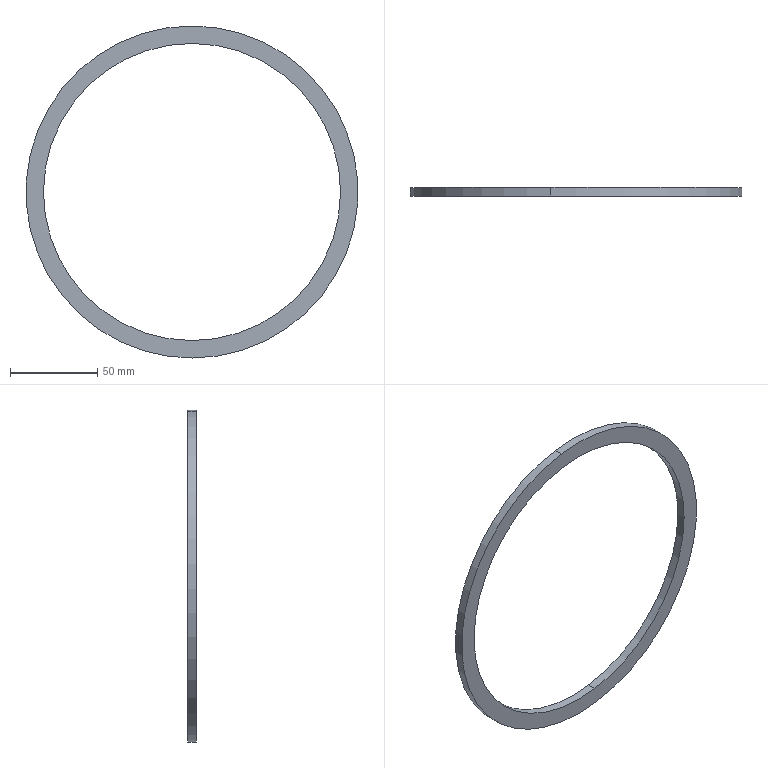Part | STEP file | 2026.6.15-Main Assembly图.sldasm-Part-10 | 1 solid | 6 faces | box 190 x 5 x 190 mm | volume 28274 mm3 | cylinder 4 | plane 2 | commonest cylinder face diameters 170 x2 190 x2
STEP:
#1=CARTESIAN_POINT('',(-741.485,695.541,3110.617));
#2=VERTEX_POINT('',#1);
#3=CARTESIAN_POINT('',(-767.19,695.541,3278.663));
#4=VERTEX_POINT('',#3);
#5=CARTESIAN_POINT('',(-754.337,695.541,3194.64));
#6=DIRECTION('',(0.,1.,0.));
#7=DIRECTION('',(-0.1512,0.,0.9885));
#8=AXIS2_PLACEMENT_3D('',#5,#6,#7);
#9=CIRCLE('',#8,85.);
#10=EDGE_CURVE('',#2,#4,#9,.T.);
#11=ORIENTED_EDGE('',*,*,#10,.T.);
#12=CARTESIAN_POINT('',(-767.19,690.541,3278.663));
#13=VERTEX_POINT('',#12);
#14=CARTESIAN_POINT('',(-767.19,695.541,3278.663));
#15=DIRECTION('',(0.,1.,0.));
#16=VECTOR('',#15,1000.);
#17=LINE('',#14,#16);
#18=EDGE_CURVE('',#13,#4,#17,.T.);
#19=ORIENTED_EDGE('',*,*,#18,.F.);
#20=CARTESIAN_POINT('',(-741.485,690.541,3110.617));
#21=VERTEX_POINT('',#20);
#22=CARTESIAN_POINT('',(-754.337,690.541,3194.64));
#23=DIRECTION('',(0.,1.,0.));
#24=DIRECTION('',(-0.1512,0.,0.9885));
#25=AXIS2_PLACEMENT_3D('',#22,#23,#24);
#26=CIRCLE('',#25,85.);
#27=EDGE_CURVE('',#21,#13,#26,.T.);
#28=ORIENTED_EDGE('',*,*,#27,.F.);
#29=CARTESIAN_POINT('',(-741.485,695.541,3110.617));
#30=DIRECTION('',(0.,1.,0.));
#31=VECTOR('',#30,1000.);
#32=LINE('',#29,#31);
#33=EDGE_CURVE('',#21,#2,#32,.T.);
#34=ORIENTED_EDGE('',*,*,#33,.T.);
#35=EDGE_LOOP('',(#11,#19,#28,#34));
#36=FACE_OUTER_BOUND('',#35,.T.);
#37=CARTESIAN_POINT('',(-754.337,695.541,3194.64));
#38=DIRECTION('',(0.,-1.,0.));
#39=DIRECTION('',(-0.1512,0.,0.9885));
#40=AXIS2_PLACEMENT_3D('',#37,#38,#39);
#41=CYLINDRICAL_SURFACE('',#40,85.);
#42=ADVANCED_FACE('',(#36),#41,.F.);
#43=CARTESIAN_POINT('',(-768.702,695.541,3288.548));
#44=VERTEX_POINT('',#43);
#45=CARTESIAN_POINT('',(-739.973,695.541,3100.732));
#46=VERTEX_POINT('',#45);
#47=CARTESIAN_POINT('',(-754.337,695.541,3194.64));
#48=DIRECTION('',(0.,1.,0.));
#49=DIRECTION('',(-0.1512,0.,0.9885));
#50=AXIS2_PLACEMENT_3D('',#47,#48,#49);
#51=CIRCLE('',#50,95.);
#52=EDGE_CURVE('',#44,#46,#51,.T.);
#53=ORIENTED_EDGE('',*,*,#52,.F.);
#54=CARTESIAN_POINT('',(-768.702,690.541,3288.548));
#55=VERTEX_POINT('',#54);
#56=CARTESIAN_POINT('',(-768.702,695.541,3288.548));
#57=DIRECTION('',(0.,1.,0.));
#58=VECTOR('',#57,1000.);
#59=LINE('',#56,#58);
#60=EDGE_CURVE('',#55,#44,#59,.T.);
#61=ORIENTED_EDGE('',*,*,#60,.F.);
#62=CARTESIAN_POINT('',(-739.973,690.541,3100.732));
#63=VERTEX_POINT('',#62);
#64=CARTESIAN_POINT('',(-754.337,690.541,3194.64));
#65=DIRECTION('',(0.,1.,0.));
#66=DIRECTION('',(-0.1512,0.,0.9885));
#67=AXIS2_PLACEMENT_3D('',#64,#65,#66);
#68=CIRCLE('',#67,95.);
#69=EDGE_CURVE('',#55,#63,#68,.T.);
#70=ORIENTED_EDGE('',*,*,#69,.T.);
#71=CARTESIAN_POINT('',(-739.973,695.541,3100.732));
#72=DIRECTION('',(0.,1.,0.));
#73=VECTOR('',#72,1000.);
#74=LINE('',#71,#73);
#75=EDGE_CURVE('',#63,#46,#74,.T.);
#76=ORIENTED_EDGE('',*,*,#75,.T.);
#77=EDGE_LOOP('',(#53,#61,#70,#76));
#78=FACE_OUTER_BOUND('',#77,.T.);
#79=CARTESIAN_POINT('',(-754.337,695.541,3194.64));
#80=DIRECTION('',(0.,-1.,0.));
#81=DIRECTION('',(-0.1512,0.,0.9885));
#82=AXIS2_PLACEMENT_3D('',#79,#80,#81);
#83=CYLINDRICAL_SURFACE('',#82,95.);
#84=ADVANCED_FACE('',(#78),#83,.T.);
#85=CARTESIAN_POINT('',(-754.337,695.541,3194.64));
#86=DIRECTION('',(0.,1.,0.));
#87=DIRECTION('',(-0.1512,0.,0.9885));
#88=AXIS2_PLACEMENT_3D('',#85,#86,#87);
#89=CIRCLE('',#88,95.);
#90=EDGE_CURVE('',#46,#44,#89,.T.);
#91=ORIENTED_EDGE('',*,*,#90,.T.);
#92=ORIENTED_EDGE('',*,*,#52,.T.);
#93=EDGE_LOOP('',(#91,#92));
#94=FACE_OUTER_BOUND('',#93,.T.);
#95=ORIENTED_EDGE('',*,*,#10,.F.);
#96=CARTESIAN_POINT('',(-754.337,695.541,3194.64));
#97=DIRECTION('',(0.,1.,0.));
#98=DIRECTION('',(-0.1512,0.,0.9885));
#99=AXIS2_PLACEMENT_3D('',#96,#97,#98);
#100=CIRCLE('',#99,85.);
#101=EDGE_CURVE('',#4,#2,#100,.T.);
#102=ORIENTED_EDGE('',*,*,#101,.F.);
#103=EDGE_LOOP('',(#95,#102));
#104=FACE_BOUND('',#103,.T.);
#105=CARTESIAN_POINT('',(-754.337,695.541,3194.64));
#106=DIRECTION('',(0.,1.,0.));
#107=DIRECTION('',(0.1512,0.,-0.9885));
#108=AXIS2_PLACEMENT_3D('',#105,#106,#107);
#109=PLANE('',#108);
#110=ADVANCED_FACE('',(#94,#104),#109,.T.);
#111=CARTESIAN_POINT('',(-754.337,690.541,3194.64));
#112=DIRECTION('',(0.,1.,0.));
#113=DIRECTION('',(-0.1512,0.,0.9885));
#114=AXIS2_PLACEMENT_3D('',#111,#112,#113);
#115=CIRCLE('',#114,95.);
#116=EDGE_CURVE('',#63,#55,#115,.T.);
#117=ORIENTED_EDGE('',*,*,#116,.F.);
#118=ORIENTED_EDGE('',*,*,#69,.F.);
#119=EDGE_LOOP('',(#117,#118));
#120=FACE_OUTER_BOUND('',#119,.T.);
#121=ORIENTED_EDGE('',*,*,#27,.T.);
#122=CARTESIAN_POINT('',(-754.337,690.541,3194.64));
#123=DIRECTION('',(0.,1.,0.));
#124=DIRECTION('',(-0.1512,0.,0.9885));
#125=AXIS2_PLACEMENT_3D('',#122,#123,#124);
#126=CIRCLE('',#125,85.);
#127=EDGE_CURVE('',#13,#21,#126,.T.);
#128=ORIENTED_EDGE('',*,*,#127,.T.);
#129=EDGE_LOOP('',(#121,#128));
#130=FACE_BOUND('',#129,.T.);
#131=CARTESIAN_POINT('',(-754.337,690.541,3194.64));
#132=DIRECTION('',(0.,1.,0.));
#133=DIRECTION('',(0.1512,0.,-0.9885));
#134=AXIS2_PLACEMENT_3D('',#131,#132,#133);
#135=PLANE('',#134);
#136=ADVANCED_FACE('',(#120,#130),#135,.F.);
#137=ORIENTED_EDGE('',*,*,#60,.T.);
#138=ORIENTED_EDGE('',*,*,#90,.F.);
#139=ORIENTED_EDGE('',*,*,#75,.F.);
#140=ORIENTED_EDGE('',*,*,#116,.T.);
#141=EDGE_LOOP('',(#137,#138,#139,#140));
#142=FACE_OUTER_BOUND('',#141,.T.);
#143=CARTESIAN_POINT('',(-754.337,695.541,3194.64));
#144=DIRECTION('',(0.,-1.,0.));
#145=DIRECTION('',(-0.1512,0.,0.9885));
#146=AXIS2_PLACEMENT_3D('',#143,#144,#145);
#147=CYLINDRICAL_SURFACE('',#146,95.);
#148=ADVANCED_FACE('',(#142),#147,.T.);
#149=ORIENTED_EDGE('',*,*,#18,.T.);
#150=ORIENTED_EDGE('',*,*,#101,.T.);
#151=ORIENTED_EDGE('',*,*,#33,.F.);
#152=ORIENTED_EDGE('',*,*,#127,.F.);
#153=EDGE_LOOP('',(#149,#150,#151,#152));
#154=FACE_OUTER_BOUND('',#153,.T.);
#155=CARTESIAN_POINT('',(-754.337,695.541,3194.64));
#156=DIRECTION('',(0.,-1.,0.));
#157=DIRECTION('',(-0.1512,0.,0.9885));
#158=AXIS2_PLACEMENT_3D('',#155,#156,#157);
#159=CYLINDRICAL_SURFACE('',#158,85.);
#160=ADVANCED_FACE('',(#154),#159,.F.);
#161=CLOSED_SHELL('',(#42,#84,#110,#136,#148,#160));
#162=MANIFOLD_SOLID_BREP('',#161);
#163=CARTESIAN_POINT('',(0.,0.,0.));
#164=DIRECTION('',(0.,0.,1.));
#165=DIRECTION('',(1.,0.,0.));
#166=AXIS2_PLACEMENT_3D('',#163,#164,#165);
#167=(LENGTH_UNIT()NAMED_UNIT(*)SI_UNIT(.MILLI.,.METRE.));
#168=UNCERTAINTY_MEASURE_WITH_UNIT(LENGTH_MEASURE(0.00001),#167,'','');
#169=(NAMED_UNIT(*)PLANE_ANGLE_UNIT()SI_UNIT($,.RADIAN.));
#170=(NAMED_UNIT(*)SI_UNIT($,.STERADIAN.)SOLID_ANGLE_UNIT());
#171=(GEOMETRIC_REPRESENTATION_CONTEXT(3)GLOBAL_UNCERTAINTY_ASSIGNED_CONTEXT((#168))GLOBAL_UNIT_ASSIGNED_CONTEXT((#167,#169,#170))REPRESENTATION_CONTEXT('',''));
#172=ADVANCED_BREP_SHAPE_REPRESENTATION('',(#162,#166),#171);